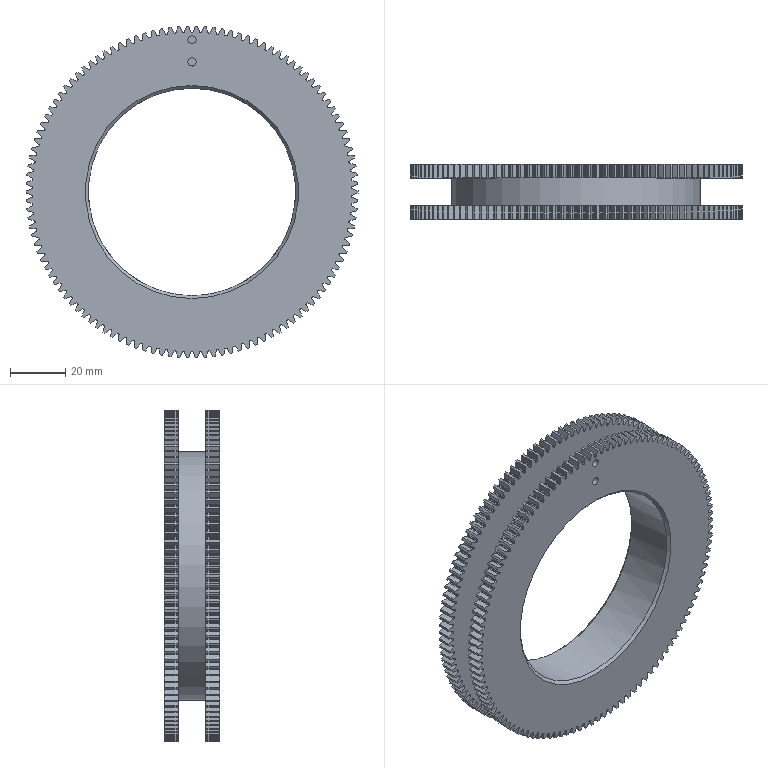Part | NX | features BREP 118, META 118, DATUM_CSYS 3, EXTRUDE 2, SKETCH 2, CHAMFER 1, CYLINDER 1, FSET 1, HOLE PACKAGE 1, SIMPLE HOLE 1 | 1 solid | 1426 faces | box 120 x 20 x 119.976 mm | volume 84081 mm3 | spline 1180 | cylinder 240 | plane 4 | cone 2 | commonest cylinder face diameters 115.5 x236 3 x2 75 x1 90 x1